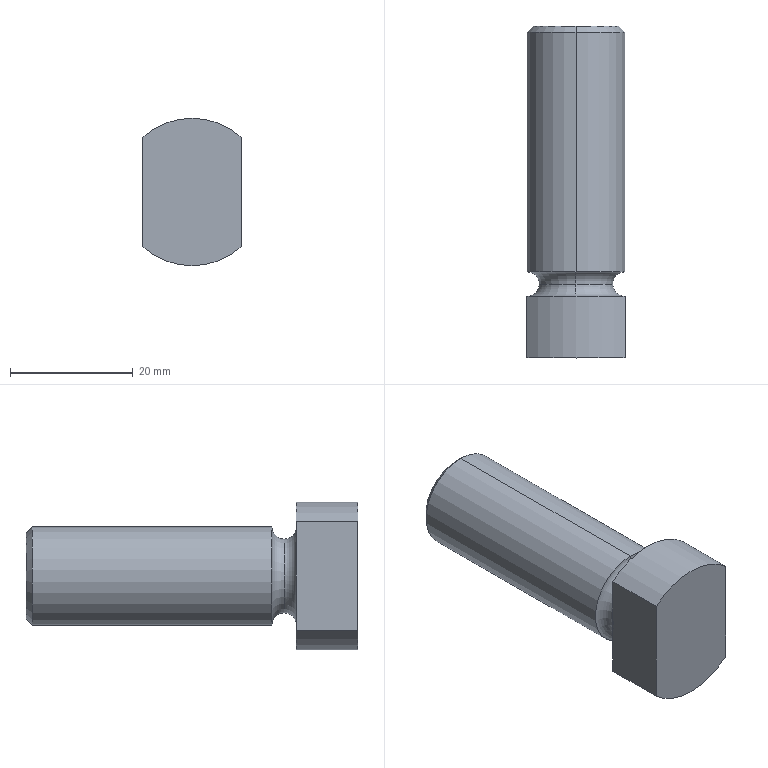Part | 1 solid | 21 faces | box 16 x 54 x 24 mm | volume 11331 mm3 | cylinder 7 | plane 6 | torus 4 | cone 4 | commonest cylinder face diameters 24 x3 6.8 x2 16 x2
STEP:
#1=CARTESIAN_POINT('',(0.,14.,8.));
#2=VERTEX_POINT('',#1);
#3=CARTESIAN_POINT('',(0.,12.,6.));
#4=VERTEX_POINT('',#3);
#5=CARTESIAN_POINT('',(0.,12.,8.));
#6=DIRECTION('',(-1.,0.,0.));
#7=DIRECTION('',(0.,0.,1.));
#8=AXIS2_PLACEMENT_3D('',#5,#6,#7);
#9=CIRCLE('',#8,2.);
#10=EDGE_CURVE('',#2,#4,#9,.T.);
#11=ORIENTED_EDGE('',*,*,#10,.T.);
#12=CARTESIAN_POINT('',(0.,12.,-6.));
#13=VERTEX_POINT('',#12);
#14=CARTESIAN_POINT('',(0.,12.,0.));
#15=DIRECTION('',(0.,1.,0.));
#16=DIRECTION('',(0.,0.,1.));
#17=AXIS2_PLACEMENT_3D('',#14,#15,#16);
#18=CIRCLE('',#17,6.);
#19=EDGE_CURVE('',#4,#13,#18,.T.);
#20=ORIENTED_EDGE('',*,*,#19,.T.);
#21=CARTESIAN_POINT('',(0.,14.,-8.));
#22=VERTEX_POINT('',#21);
#23=CARTESIAN_POINT('',(0.,12.,-8.));
#24=DIRECTION('',(1.,0.,0.));
#25=DIRECTION('',(0.,0.,-1.));
#26=AXIS2_PLACEMENT_3D('',#23,#24,#25);
#27=CIRCLE('',#26,2.);
#28=EDGE_CURVE('',#22,#13,#27,.T.);
#29=ORIENTED_EDGE('',*,*,#28,.F.);
#30=CARTESIAN_POINT('',(0.,14.,0.));
#31=DIRECTION('',(0.,1.,0.));
#32=DIRECTION('',(0.,0.,-1.));
#33=AXIS2_PLACEMENT_3D('',#30,#31,#32);
#34=CIRCLE('',#33,8.);
#35=EDGE_CURVE('',#2,#22,#34,.T.);
#36=ORIENTED_EDGE('',*,*,#35,.F.);
#37=EDGE_LOOP('',(#11,#20,#29,#36));
#38=FACE_OUTER_BOUND('',#37,.T.);
#39=CARTESIAN_POINT('',(0.,12.,0.));
#40=DIRECTION('',(0.,1.,0.));
#41=DIRECTION('',(0.,0.,1.));
#42=AXIS2_PLACEMENT_3D('',#39,#40,#41);
#43=TOROIDAL_SURFACE('',#42,8.,2.);
#44=ADVANCED_FACE('',(#38),#43,.F.);
#45=ORIENTED_EDGE('',*,*,#28,.T.);
#46=CARTESIAN_POINT('',(0.,12.,0.));
#47=DIRECTION('',(0.,1.,0.));
#48=DIRECTION('',(0.,0.,1.));
#49=AXIS2_PLACEMENT_3D('',#46,#47,#48);
#50=CIRCLE('',#49,6.);
#51=EDGE_CURVE('',#13,#4,#50,.T.);
#52=ORIENTED_EDGE('',*,*,#51,.T.);
#53=ORIENTED_EDGE('',*,*,#10,.F.);
#54=CARTESIAN_POINT('',(0.,14.,0.));
#55=DIRECTION('',(0.,1.,0.));
#56=DIRECTION('',(0.,0.,-1.));
#57=AXIS2_PLACEMENT_3D('',#54,#55,#56);
#58=CIRCLE('',#57,8.);
#59=EDGE_CURVE('',#22,#2,#58,.T.);
#60=ORIENTED_EDGE('',*,*,#59,.F.);
#61=EDGE_LOOP('',(#45,#52,#53,#60));
#62=FACE_OUTER_BOUND('',#61,.T.);
#63=CARTESIAN_POINT('',(0.,12.,0.));
#64=DIRECTION('',(0.,1.,0.));
#65=DIRECTION('',(0.,0.,1.));
#66=AXIS2_PLACEMENT_3D('',#63,#64,#65);
#67=TOROIDAL_SURFACE('',#66,8.,2.);
#68=ADVANCED_FACE('',(#62),#67,.F.);
#69=CARTESIAN_POINT('',(0.,10.,-12.));
#70=VERTEX_POINT('',#69);
#71=CARTESIAN_POINT('',(-8.,10.,-8.944));
#72=VERTEX_POINT('',#71);
#73=CARTESIAN_POINT('',(0.,10.,0.));
#74=DIRECTION('',(0.,1.,0.));
#75=DIRECTION('',(0.,0.,1.));
#76=AXIS2_PLACEMENT_3D('',#73,#74,#75);
#77=CIRCLE('',#76,12.);
#78=EDGE_CURVE('',#70,#72,#77,.T.);
#79=ORIENTED_EDGE('',*,*,#78,.F.);
#80=CARTESIAN_POINT('',(0.,0.,-12.));
#81=VERTEX_POINT('',#80);
#82=CARTESIAN_POINT('',(0.,10.,-12.));
#83=DIRECTION('',(0.,-1.,0.));
#84=VECTOR('',#83,1000.);
#85=LINE('',#82,#84);
#86=EDGE_CURVE('',#70,#81,#85,.T.);
#87=ORIENTED_EDGE('',*,*,#86,.T.);
#88=CARTESIAN_POINT('',(-8.,0.,-8.944));
#89=VERTEX_POINT('',#88);
#90=CARTESIAN_POINT('',(0.,0.,0.));
#91=DIRECTION('',(0.,1.,0.));
#92=DIRECTION('',(0.,0.,1.));
#93=AXIS2_PLACEMENT_3D('',#90,#91,#92);
#94=CIRCLE('',#93,12.);
#95=EDGE_CURVE('',#81,#89,#94,.T.);
#96=ORIENTED_EDGE('',*,*,#95,.T.);
#97=CARTESIAN_POINT('',(-8.,-34.,-8.944));
#98=DIRECTION('',(0.,1.,0.));
#99=VECTOR('',#98,1000.);
#100=LINE('',#97,#99);
#101=EDGE_CURVE('',#89,#72,#100,.T.);
#102=ORIENTED_EDGE('',*,*,#101,.T.);
#103=EDGE_LOOP('',(#79,#87,#96,#102));
#104=FACE_OUTER_BOUND('',#103,.T.);
#105=CARTESIAN_POINT('',(0.,10.,0.));
#106=DIRECTION('',(0.,-1.,0.));
#107=DIRECTION('',(0.,0.,-1.));
#108=AXIS2_PLACEMENT_3D('',#105,#106,#107);
#109=CYLINDRICAL_SURFACE('',#108,12.);
#110=ADVANCED_FACE('',(#104),#109,.T.);
#111=ORIENTED_EDGE('',*,*,#51,.F.);
#112=CARTESIAN_POINT('',(0.,10.,-8.));
#113=VERTEX_POINT('',#112);
#114=CARTESIAN_POINT('',(0.,12.,-8.));
#115=DIRECTION('',(1.,0.,0.));
#116=DIRECTION('',(0.,0.,-1.));
#117=AXIS2_PLACEMENT_3D('',#114,#115,#116);
#118=CIRCLE('',#117,2.);
#119=EDGE_CURVE('',#13,#113,#118,.T.);
#120=ORIENTED_EDGE('',*,*,#119,.T.);
#121=CARTESIAN_POINT('',(-8.,10.,0.));
#122=VERTEX_POINT('',#121);
#123=CARTESIAN_POINT('',(0.,10.,0.));
#124=DIRECTION('',(0.,1.,0.));
#125=DIRECTION('',(0.,0.,1.));
#126=AXIS2_PLACEMENT_3D('',#123,#124,#125);
#127=CIRCLE('',#126,8.);
#128=EDGE_CURVE('',#113,#122,#127,.T.);
#129=ORIENTED_EDGE('',*,*,#128,.T.);
#130=CARTESIAN_POINT('',(0.,10.,8.));
#131=VERTEX_POINT('',#130);
#132=CARTESIAN_POINT('',(0.,10.,0.));
#133=DIRECTION('',(0.,1.,0.));
#134=DIRECTION('',(0.,0.,1.));
#135=AXIS2_PLACEMENT_3D('',#132,#133,#134);
#136=CIRCLE('',#135,8.);
#137=EDGE_CURVE('',#122,#131,#136,.T.);
#138=ORIENTED_EDGE('',*,*,#137,.T.);
#139=CARTESIAN_POINT('',(0.,12.,8.));
#140=DIRECTION('',(-1.,0.,0.));
#141=DIRECTION('',(0.,0.,1.));
#142=AXIS2_PLACEMENT_3D('',#139,#140,#141);
#143=CIRCLE('',#142,2.);
#144=EDGE_CURVE('',#4,#131,#143,.T.);
#145=ORIENTED_EDGE('',*,*,#144,.F.);
#146=EDGE_LOOP('',(#111,#120,#129,#138,#145));
#147=FACE_OUTER_BOUND('',#146,.T.);
#148=CARTESIAN_POINT('',(0.,12.,0.));
#149=DIRECTION('',(0.,1.,0.));
#150=DIRECTION('',(0.,0.,1.));
#151=AXIS2_PLACEMENT_3D('',#148,#149,#150);
#152=TOROIDAL_SURFACE('',#151,8.,2.);
#153=ADVANCED_FACE('',(#147),#152,.F.);
#154=CARTESIAN_POINT('',(0.,54.,7.));
#155=VERTEX_POINT('',#154);
#156=CARTESIAN_POINT('',(0.,54.,-7.));
#157=VERTEX_POINT('',#156);
#158=CARTESIAN_POINT('',(0.,54.,0.));
#159=DIRECTION('',(0.,1.,0.));
#160=DIRECTION('',(0.,0.,1.));
#161=AXIS2_PLACEMENT_3D('',#158,#159,#160);
#162=CIRCLE('',#161,7.);
#163=EDGE_CURVE('',#155,#157,#162,.T.);
#164=ORIENTED_EDGE('',*,*,#163,.F.);
#165=CARTESIAN_POINT('',(0.,53.,8.));
#166=VERTEX_POINT('',#165);
#167=CARTESIAN_POINT('',(0.,54.,7.));
#168=DIRECTION('',(0.,-0.7071,0.7071));
#169=VECTOR('',#168,1000.);
#170=LINE('',#167,#169);
#171=EDGE_CURVE('',#155,#166,#170,.T.);
#172=ORIENTED_EDGE('',*,*,#171,.T.);
#173=CARTESIAN_POINT('',(0.,53.,-8.));
#174=VERTEX_POINT('',#173);
#175=CARTESIAN_POINT('',(0.,53.,0.));
#176=DIRECTION('',(0.,-1.,0.));
#177=DIRECTION('',(0.,0.,1.));
#178=AXIS2_PLACEMENT_3D('',#175,#176,#177);
#179=CIRCLE('',#178,8.);
#180=EDGE_CURVE('',#174,#166,#179,.T.);
#181=ORIENTED_EDGE('',*,*,#180,.F.);
#182=CARTESIAN_POINT('',(0.,54.,-7.));
#183=DIRECTION('',(0.,-0.7071,-0.7071));
#184=VECTOR('',#183,1000.);
#185=LINE('',#182,#184);
#186=EDGE_CURVE('',#157,#174,#185,.T.);
#187=ORIENTED_EDGE('',*,*,#186,.F.);
#188=EDGE_LOOP('',(#164,#172,#181,#187));
#189=FACE_OUTER_BOUND('',#188,.T.);
#190=CARTESIAN_POINT('',(0.,54.,0.));
#191=DIRECTION('',(0.,-1.,0.));
#192=DIRECTION('',(0.,0.,-1.));
#193=AXIS2_PLACEMENT_3D('',#190,#191,#192);
#194=CONICAL_SURFACE('',#193,7.,0.7854);
#195=ADVANCED_FACE('',(#189),#194,.T.);
#196=CARTESIAN_POINT('',(0.,34.25,-3.4));
#197=VERTEX_POINT('',#196);
#198=CARTESIAN_POINT('',(0.,34.25,3.4));
#199=VERTEX_POINT('',#198);
#200=CARTESIAN_POINT('',(0.,34.25,0.));
#201=DIRECTION('',(0.,1.,0.));
#202=DIRECTION('',(0.,0.,1.));
#203=AXIS2_PLACEMENT_3D('',#200,#201,#202);
#204=CIRCLE('',#203,3.4);
#205=EDGE_CURVE('',#197,#199,#204,.T.);
#206=ORIENTED_EDGE('',*,*,#205,.F.);
#207=CARTESIAN_POINT('',(0.,54.,-3.4));
#208=VERTEX_POINT('',#207);
#209=CARTESIAN_POINT('',(0.,54.,-3.4));
#210=DIRECTION('',(0.,1.,0.));
#211=VECTOR('',#210,1000.);
#212=LINE('',#209,#211);
#213=EDGE_CURVE('',#197,#208,#212,.T.);
#214=ORIENTED_EDGE('',*,*,#213,.T.);
#215=CARTESIAN_POINT('',(0.,54.,3.4));
#216=VERTEX_POINT('',#215);
#217=CARTESIAN_POINT('',(0.,54.,0.));
#218=DIRECTION('',(0.,1.,0.));
#219=DIRECTION('',(0.,0.,1.));
#220=AXIS2_PLACEMENT_3D('',#217,#218,#219);
#221=CIRCLE('',#220,3.4);
#222=EDGE_CURVE('',#208,#216,#221,.T.);
#223=ORIENTED_EDGE('',*,*,#222,.T.);
#224=CARTESIAN_POINT('',(0.,54.,3.4));
#225=DIRECTION('',(0.,1.,0.));
#226=VECTOR('',#225,1000.);
#227=LINE('',#224,#226);
#228=EDGE_CURVE('',#199,#216,#227,.T.);
#229=ORIENTED_EDGE('',*,*,#228,.F.);
#230=EDGE_LOOP('',(#206,#214,#223,#229));
#231=FACE_OUTER_BOUND('',#230,.T.);
#232=CARTESIAN_POINT('',(0.,54.,0.));
#233=DIRECTION('',(0.,1.,0.));
#234=DIRECTION('',(0.,0.,1.));
#235=AXIS2_PLACEMENT_3D('',#232,#233,#234);
#236=CYLINDRICAL_SURFACE('',#235,3.4);
#237=ADVANCED_FACE('',(#231),#236,.F.);
#238=CARTESIAN_POINT('',(0.,32.207,0.));
#239=VERTEX_POINT('',#238);
#240=CARTESIAN_POINT('',(0.,34.25,3.4));
#241=DIRECTION('',(0.,0.515,0.8572));
#242=VECTOR('',#241,1000.);
#243=LINE('',#240,#242);
#244=EDGE_CURVE('',#239,#199,#243,.T.);
#245=ORIENTED_EDGE('',*,*,#244,.F.);
#246=CARTESIAN_POINT('',(0.,34.25,-3.4));
#247=DIRECTION('',(0.,0.515,-0.8572));
#248=VECTOR('',#247,1000.);
#249=LINE('',#246,#248);
#250=EDGE_CURVE('',#239,#197,#249,.T.);
#251=ORIENTED_EDGE('',*,*,#250,.T.);
#252=ORIENTED_EDGE('',*,*,#205,.T.);
#253=EDGE_LOOP('',(#245,#251,#252));
#254=FACE_OUTER_BOUND('',#253,.T.);
#255=CARTESIAN_POINT('',(0.,34.25,0.));
#256=DIRECTION('',(0.,1.,0.));
#257=DIRECTION('',(0.,0.,1.));
#258=AXIS2_PLACEMENT_3D('',#255,#256,#257);
#259=CONICAL_SURFACE('',#258,3.4,1.03);
#260=ADVANCED_FACE('',(#254),#259,.F.);
#261=ORIENTED_EDGE('',*,*,#180,.T.);
#262=CARTESIAN_POINT('',(0.,54.,8.));
#263=DIRECTION('',(0.,-1.,0.));
#264=VECTOR('',#263,1000.);
#265=LINE('',#262,#264);
#266=EDGE_CURVE('',#166,#2,#265,.T.);
#267=ORIENTED_EDGE('',*,*,#266,.T.);
#268=ORIENTED_EDGE('',*,*,#35,.T.);
#269=CARTESIAN_POINT('',(0.,54.,-8.));
#270=DIRECTION('',(0.,-1.,0.));
#271=VECTOR('',#270,1000.);
#272=LINE('',#269,#271);
#273=EDGE_CURVE('',#174,#22,#272,.T.);
#274=ORIENTED_EDGE('',*,*,#273,.F.);
#275=EDGE_LOOP('',(#261,#267,#268,#274));
#276=FACE_OUTER_BOUND('',#275,.T.);
#277=CARTESIAN_POINT('',(0.,54.,0.));
#278=DIRECTION('',(0.,-1.,0.));
#279=DIRECTION('',(0.,0.,-1.));
#280=AXIS2_PLACEMENT_3D('',#277,#278,#279);
#281=CYLINDRICAL_SURFACE('',#280,8.);
#282=ADVANCED_FACE('',(#276),#281,.T.);
#283=ORIENTED_EDGE('',*,*,#266,.F.);
#284=CARTESIAN_POINT('',(0.,53.,0.));
#285=DIRECTION('',(0.,-1.,0.));
#286=DIRECTION('',(0.,0.,1.));
#287=AXIS2_PLACEMENT_3D('',#284,#285,#286);
#288=CIRCLE('',#287,8.);
#289=EDGE_CURVE('',#166,#174,#288,.T.);
#290=ORIENTED_EDGE('',*,*,#289,.T.);
#291=ORIENTED_EDGE('',*,*,#273,.T.);
#292=ORIENTED_EDGE('',*,*,#59,.T.);
#293=EDGE_LOOP('',(#283,#290,#291,#292));
#294=FACE_OUTER_BOUND('',#293,.T.);
#295=CARTESIAN_POINT('',(0.,54.,0.));
#296=DIRECTION('',(0.,-1.,0.));
#297=DIRECTION('',(0.,0.,-1.));
#298=AXIS2_PLACEMENT_3D('',#295,#296,#297);
#299=CYLINDRICAL_SURFACE('',#298,8.);
#300=ADVANCED_FACE('',(#294),#299,.T.);
#301=CARTESIAN_POINT('',(0.,54.,0.));
#302=DIRECTION('',(0.,1.,0.));
#303=DIRECTION('',(0.,0.,1.));
#304=AXIS2_PLACEMENT_3D('',#301,#302,#303);
#305=CIRCLE('',#304,7.);
#306=EDGE_CURVE('',#157,#155,#305,.T.);
#307=ORIENTED_EDGE('',*,*,#306,.T.);
#308=ORIENTED_EDGE('',*,*,#163,.T.);
#309=EDGE_LOOP('',(#307,#308));
#310=FACE_OUTER_BOUND('',#309,.T.);
#311=CARTESIAN_POINT('',(0.,54.,0.));
#312=DIRECTION('',(0.,1.,0.));
#313=DIRECTION('',(0.,0.,1.));
#314=AXIS2_PLACEMENT_3D('',#311,#312,#313);
#315=CIRCLE('',#314,3.4);
#316=EDGE_CURVE('',#216,#208,#315,.T.);
#317=ORIENTED_EDGE('',*,*,#316,.F.);
#318=ORIENTED_EDGE('',*,*,#222,.F.);
#319=EDGE_LOOP('',(#317,#318));
#320=FACE_BOUND('',#319,.T.);
#321=CARTESIAN_POINT('',(0.,54.,0.));
#322=DIRECTION('',(0.,1.,0.));
#323=DIRECTION('',(0.,0.,1.));
#324=AXIS2_PLACEMENT_3D('',#321,#322,#323);
#325=PLANE('',#324);
#326=ADVANCED_FACE('',(#310,#320),#325,.T.);
#327=ORIENTED_EDGE('',*,*,#250,.F.);
#328=ORIENTED_EDGE('',*,*,#244,.T.);
#329=CARTESIAN_POINT('',(0.,34.25,0.));
#330=DIRECTION('',(0.,1.,0.));
#331=DIRECTION('',(0.,0.,1.));
#332=AXIS2_PLACEMENT_3D('',#329,#330,#331);
#333=CIRCLE('',#332,3.4);
#334=EDGE_CURVE('',#199,#197,#333,.T.);
#335=ORIENTED_EDGE('',*,*,#334,.T.);
#336=EDGE_LOOP('',(#327,#328,#335));
#337=FACE_OUTER_BOUND('',#336,.T.);
#338=CARTESIAN_POINT('',(0.,34.25,0.));
#339=DIRECTION('',(0.,1.,0.));
#340=DIRECTION('',(0.,0.,1.));
#341=AXIS2_PLACEMENT_3D('',#338,#339,#340);
#342=CONICAL_SURFACE('',#341,3.4,1.03);
#343=ADVANCED_FACE('',(#337),#342,.F.);
#344=ORIENTED_EDGE('',*,*,#213,.F.);
#345=ORIENTED_EDGE('',*,*,#334,.F.);
#346=ORIENTED_EDGE('',*,*,#228,.T.);
#347=ORIENTED_EDGE('',*,*,#316,.T.);
#348=EDGE_LOOP('',(#344,#345,#346,#347));
#349=FACE_OUTER_BOUND('',#348,.T.);
#350=CARTESIAN_POINT('',(0.,54.,0.));
#351=DIRECTION('',(0.,1.,0.));
#352=DIRECTION('',(0.,0.,1.));
#353=AXIS2_PLACEMENT_3D('',#350,#351,#352);
#354=CYLINDRICAL_SURFACE('',#353,3.4);
#355=ADVANCED_FACE('',(#349),#354,.F.);
#356=ORIENTED_EDGE('',*,*,#171,.F.);
#357=ORIENTED_EDGE('',*,*,#306,.F.);
#358=ORIENTED_EDGE('',*,*,#186,.T.);
#359=ORIENTED_EDGE('',*,*,#289,.F.);
#360=EDGE_LOOP('',(#356,#357,#358,#359));
#361=FACE_OUTER_BOUND('',#360,.T.);
#362=CARTESIAN_POINT('',(0.,54.,0.));
#363=DIRECTION('',(0.,-1.,0.));
#364=DIRECTION('',(0.,0.,-1.));
#365=AXIS2_PLACEMENT_3D('',#362,#363,#364);
#366=CONICAL_SURFACE('',#365,7.,0.7854);
#367=ADVANCED_FACE('',(#361),#366,.T.);
#368=ORIENTED_EDGE('',*,*,#19,.F.);
#369=ORIENTED_EDGE('',*,*,#144,.T.);
#370=CARTESIAN_POINT('',(8.,10.,0.));
#371=VERTEX_POINT('',#370);
#372=CARTESIAN_POINT('',(0.,10.,0.));
#373=DIRECTION('',(0.,1.,0.));
#374=DIRECTION('',(0.,0.,1.));
#375=AXIS2_PLACEMENT_3D('',#372,#373,#374);
#376=CIRCLE('',#375,8.);
#377=EDGE_CURVE('',#131,#371,#376,.T.);
#378=ORIENTED_EDGE('',*,*,#377,.T.);
#379=CARTESIAN_POINT('',(0.,10.,0.));
#380=DIRECTION('',(0.,1.,0.));
#381=DIRECTION('',(0.,0.,1.));
#382=AXIS2_PLACEMENT_3D('',#379,#380,#381);
#383=CIRCLE('',#382,8.);
#384=EDGE_CURVE('',#371,#113,#383,.T.);
#385=ORIENTED_EDGE('',*,*,#384,.T.);
#386=ORIENTED_EDGE('',*,*,#119,.F.);
#387=EDGE_LOOP('',(#368,#369,#378,#385,#386));
#388=FACE_OUTER_BOUND('',#387,.T.);
#389=CARTESIAN_POINT('',(0.,12.,0.));
#390=DIRECTION('',(0.,1.,0.));
#391=DIRECTION('',(0.,0.,1.));
#392=AXIS2_PLACEMENT_3D('',#389,#390,#391);
#393=TOROIDAL_SURFACE('',#392,8.,2.);
#394=ADVANCED_FACE('',(#388),#393,.F.);
#395=CARTESIAN_POINT('',(-8.,0.,8.944));
#396=VERTEX_POINT('',#395);
#397=CARTESIAN_POINT('',(8.,0.,8.944));
#398=VERTEX_POINT('',#397);
#399=CARTESIAN_POINT('',(0.,0.,0.));
#400=DIRECTION('',(0.,1.,0.));
#401=DIRECTION('',(0.,0.,1.));
#402=AXIS2_PLACEMENT_3D('',#399,#400,#401);
#403=CIRCLE('',#402,12.);
#404=EDGE_CURVE('',#396,#398,#403,.T.);
#405=ORIENTED_EDGE('',*,*,#404,.F.);
#406=CARTESIAN_POINT('',(-8.,0.,0.));
#407=DIRECTION('',(0.,0.,-1.));
#408=VECTOR('',#407,1000.);
#409=LINE('',#406,#408);
#410=EDGE_CURVE('',#396,#89,#409,.T.);
#411=ORIENTED_EDGE('',*,*,#410,.T.);
#412=ORIENTED_EDGE('',*,*,#95,.F.);
#413=CARTESIAN_POINT('',(8.,0.,-8.944));
#414=VERTEX_POINT('',#413);
#415=CARTESIAN_POINT('',(0.,0.,0.));
#416=DIRECTION('',(0.,1.,0.));
#417=DIRECTION('',(0.,0.,1.));
#418=AXIS2_PLACEMENT_3D('',#415,#416,#417);
#419=CIRCLE('',#418,12.);
#420=EDGE_CURVE('',#414,#81,#419,.T.);
#421=ORIENTED_EDGE('',*,*,#420,.F.);
#422=CARTESIAN_POINT('',(8.,0.,0.));
#423=DIRECTION('',(0.,0.,1.));
#424=VECTOR('',#423,1000.);
#425=LINE('',#422,#424);
#426=EDGE_CURVE('',#414,#398,#425,.T.);
#427=ORIENTED_EDGE('',*,*,#426,.T.);
#428=EDGE_LOOP('',(#405,#411,#412,#421,#427));
#429=FACE_OUTER_BOUND('',#428,.T.);
#430=CARTESIAN_POINT('',(0.,0.,0.));
#431=DIRECTION('',(0.,1.,0.));
#432=DIRECTION('',(0.,0.,1.));
#433=AXIS2_PLACEMENT_3D('',#430,#431,#432);
#434=PLANE('',#433);
#435=ADVANCED_FACE('',(#429),#434,.F.);
#436=ORIENTED_EDGE('',*,*,#86,.F.);
#437=CARTESIAN_POINT('',(8.,10.,-8.944));
#438=VERTEX_POINT('',#437);
#439=CARTESIAN_POINT('',(0.,10.,0.));
#440=DIRECTION('',(0.,1.,0.));
#441=DIRECTION('',(0.,0.,1.));
#442=AXIS2_PLACEMENT_3D('',#439,#440,#441);
#443=CIRCLE('',#442,12.);
#444=EDGE_CURVE('',#438,#70,#443,.T.);
#445=ORIENTED_EDGE('',*,*,#444,.F.);
#446=CARTESIAN_POINT('',(8.,-34.,-8.944));
#447=DIRECTION('',(0.,1.,0.));
#448=VECTOR('',#447,1000.);
#449=LINE('',#446,#448);
#450=EDGE_CURVE('',#414,#438,#449,.T.);
#451=ORIENTED_EDGE('',*,*,#450,.F.);
#452=ORIENTED_EDGE('',*,*,#420,.T.);
#453=EDGE_LOOP('',(#436,#445,#451,#452));
#454=FACE_OUTER_BOUND('',#453,.T.);
#455=CARTESIAN_POINT('',(0.,10.,0.));
#456=DIRECTION('',(0.,-1.,0.));
#457=DIRECTION('',(0.,0.,-1.));
#458=AXIS2_PLACEMENT_3D('',#455,#456,#457);
#459=CYLINDRICAL_SURFACE('',#458,12.);
#460=ADVANCED_FACE('',(#454),#459,.T.);
#461=ORIENTED_EDGE('',*,*,#450,.T.);
#462=CARTESIAN_POINT('',(8.,10.,-8.944));
#463=DIRECTION('',(0.,0.,1.));
#464=VECTOR('',#463,1000.);
#465=LINE('',#462,#464);
#466=EDGE_CURVE('',#438,#371,#465,.T.);
#467=ORIENTED_EDGE('',*,*,#466,.T.);
#468=CARTESIAN_POINT('',(8.,10.,8.944));
#469=VERTEX_POINT('',#468);
#470=CARTESIAN_POINT('',(8.,10.,-8.944));
#471=DIRECTION('',(0.,0.,1.));
#472=VECTOR('',#471,1000.);
#473=LINE('',#470,#472);
#474=EDGE_CURVE('',#371,#469,#473,.T.);
#475=ORIENTED_EDGE('',*,*,#474,.T.);
#476=CARTESIAN_POINT('',(8.,-34.,8.944));
#477=DIRECTION('',(0.,1.,0.));
#478=VECTOR('',#477,1000.);
#479=LINE('',#476,#478);
#480=EDGE_CURVE('',#398,#469,#479,.T.);
#481=ORIENTED_EDGE('',*,*,#480,.F.);
#482=ORIENTED_EDGE('',*,*,#426,.F.);
#483=EDGE_LOOP('',(#461,#467,#475,#481,#482));
#484=FACE_OUTER_BOUND('',#483,.T.);
#485=CARTESIAN_POINT('',(8.,-34.,-8.944));
#486=DIRECTION('',(-1.,0.,0.));
#487=DIRECTION('',(0.,0.,1.));
#488=AXIS2_PLACEMENT_3D('',#485,#486,#487);
#489=PLANE('',#488);
#490=ADVANCED_FACE('',(#484),#489,.F.);
#491=CARTESIAN_POINT('',(-8.,10.,8.944));
#492=VERTEX_POINT('',#491);
#493=CARTESIAN_POINT('',(0.,10.,0.));
#494=DIRECTION('',(0.,1.,0.));
#495=DIRECTION('',(0.,0.,1.));
#496=AXIS2_PLACEMENT_3D('',#493,#494,#495);
#497=CIRCLE('',#496,12.);
#498=EDGE_CURVE('',#492,#469,#497,.T.);
#499=ORIENTED_EDGE('',*,*,#498,.F.);
#500=CARTESIAN_POINT('',(-8.,-34.,8.944));
#501=DIRECTION('',(0.,1.,0.));
#502=VECTOR('',#501,1000.);
#503=LINE('',#500,#502);
#504=EDGE_CURVE('',#396,#492,#503,.T.);
#505=ORIENTED_EDGE('',*,*,#504,.F.);
#506=ORIENTED_EDGE('',*,*,#404,.T.);
#507=ORIENTED_EDGE('',*,*,#480,.T.);
#508=EDGE_LOOP('',(#499,#505,#506,#507));
#509=FACE_OUTER_BOUND('',#508,.T.);
#510=CARTESIAN_POINT('',(0.,10.,0.));
#511=DIRECTION('',(0.,-1.,0.));
#512=DIRECTION('',(0.,0.,-1.));
#513=AXIS2_PLACEMENT_3D('',#510,#511,#512);
#514=CYLINDRICAL_SURFACE('',#513,12.);
#515=ADVANCED_FACE('',(#509),#514,.T.);
#516=CARTESIAN_POINT('',(-8.,10.,-8.944));
#517=DIRECTION('',(0.,0.,-1.));
#518=VECTOR('',#517,1000.);
#519=LINE('',#516,#518);
#520=EDGE_CURVE('',#122,#72,#519,.T.);
#521=ORIENTED_EDGE('',*,*,#520,.F.);
#522=ORIENTED_EDGE('',*,*,#128,.F.);
#523=ORIENTED_EDGE('',*,*,#384,.F.);
#524=ORIENTED_EDGE('',*,*,#466,.F.);
#525=ORIENTED_EDGE('',*,*,#444,.T.);
#526=ORIENTED_EDGE('',*,*,#78,.T.);
#527=EDGE_LOOP('',(#521,#522,#523,#524,#525,#526));
#528=FACE_OUTER_BOUND('',#527,.T.);
#529=CARTESIAN_POINT('',(0.,10.,0.));
#530=DIRECTION('',(0.,1.,0.));
#531=DIRECTION('',(0.,0.,1.));
#532=AXIS2_PLACEMENT_3D('',#529,#530,#531);
#533=PLANE('',#532);
#534=ADVANCED_FACE('',(#528),#533,.T.);
#535=ORIENTED_EDGE('',*,*,#504,.T.);
#536=CARTESIAN_POINT('',(-8.,10.,-8.944));
#537=DIRECTION('',(0.,0.,-1.));
#538=VECTOR('',#537,1000.);
#539=LINE('',#536,#538);
#540=EDGE_CURVE('',#492,#122,#539,.T.);
#541=ORIENTED_EDGE('',*,*,#540,.T.);
#542=ORIENTED_EDGE('',*,*,#520,.T.);
#543=ORIENTED_EDGE('',*,*,#101,.F.);
#544=ORIENTED_EDGE('',*,*,#410,.F.);
#545=EDGE_LOOP('',(#535,#541,#542,#543,#544));
#546=FACE_OUTER_BOUND('',#545,.T.);
#547=CARTESIAN_POINT('',(-8.,-34.,-8.944));
#548=DIRECTION('',(1.,0.,0.));
#549=DIRECTION('',(0.,0.,-1.));
#550=AXIS2_PLACEMENT_3D('',#547,#548,#549);
#551=PLANE('',#550);
#552=ADVANCED_FACE('',(#546),#551,.F.);
#553=ORIENTED_EDGE('',*,*,#540,.F.);
#554=ORIENTED_EDGE('',*,*,#498,.T.);
#555=ORIENTED_EDGE('',*,*,#474,.F.);
#556=ORIENTED_EDGE('',*,*,#377,.F.);
#557=ORIENTED_EDGE('',*,*,#137,.F.);
#558=EDGE_LOOP('',(#553,#554,#555,#556,#557));
#559=FACE_OUTER_BOUND('',#558,.T.);
#560=CARTESIAN_POINT('',(0.,10.,0.));
#561=DIRECTION('',(0.,1.,0.));
#562=DIRECTION('',(0.,0.,1.));
#563=AXIS2_PLACEMENT_3D('',#560,#561,#562);
#564=PLANE('',#563);
#565=ADVANCED_FACE('',(#559),#564,.T.);
#566=CLOSED_SHELL('',(#44,#68,#110,#153,#195,#237,#260,#282,#300,#326,#343,#355,#367,#394,#435,#460,#490,#515,#534,#552,#565));
#567=MANIFOLD_SOLID_BREP('',#566);
#568=CARTESIAN_POINT('',(0.,0.,0.));
#569=DIRECTION('',(0.,0.,1.));
#570=DIRECTION('',(1.,0.,0.));
#571=AXIS2_PLACEMENT_3D('',#568,#569,#570);
#572=(LENGTH_UNIT()NAMED_UNIT(*)SI_UNIT(.MILLI.,.METRE.));
#573=UNCERTAINTY_MEASURE_WITH_UNIT(LENGTH_MEASURE(0.00001),#572,'','');
#574=(NAMED_UNIT(*)PLANE_ANGLE_UNIT()SI_UNIT($,.RADIAN.));
#575=(NAMED_UNIT(*)SI_UNIT($,.STERADIAN.)SOLID_ANGLE_UNIT());
#576=(GEOMETRIC_REPRESENTATION_CONTEXT(3)GLOBAL_UNCERTAINTY_ASSIGNED_CONTEXT((#573))GLOBAL_UNIT_ASSIGNED_CONTEXT((#572,#574,#575))REPRESENTATION_CONTEXT('',''));
#577=ADVANCED_BREP_SHAPE_REPRESENTATION('',(#567,#571),#576);